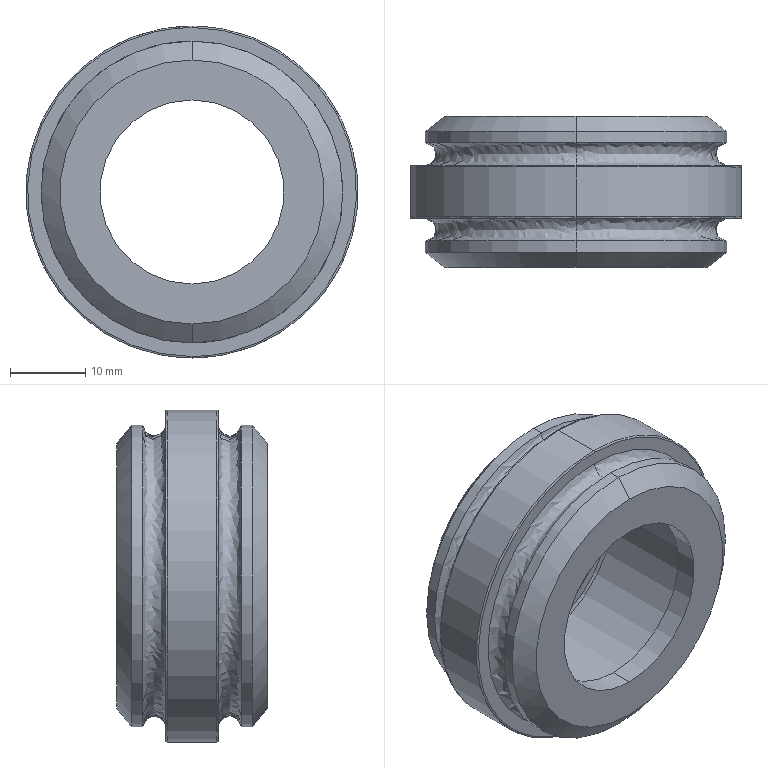Part | SolidWorks | features BaseBody 1 | 1 solid | 33 faces | box 44 x 20 x 44 mm | volume 13523 mm3 | cylinder 14 | spline 8 | plane 7 | cone 4 | commonest cylinder face diameters 28 x4 40 x4 24.4 x2 30.1 x2 44 x2